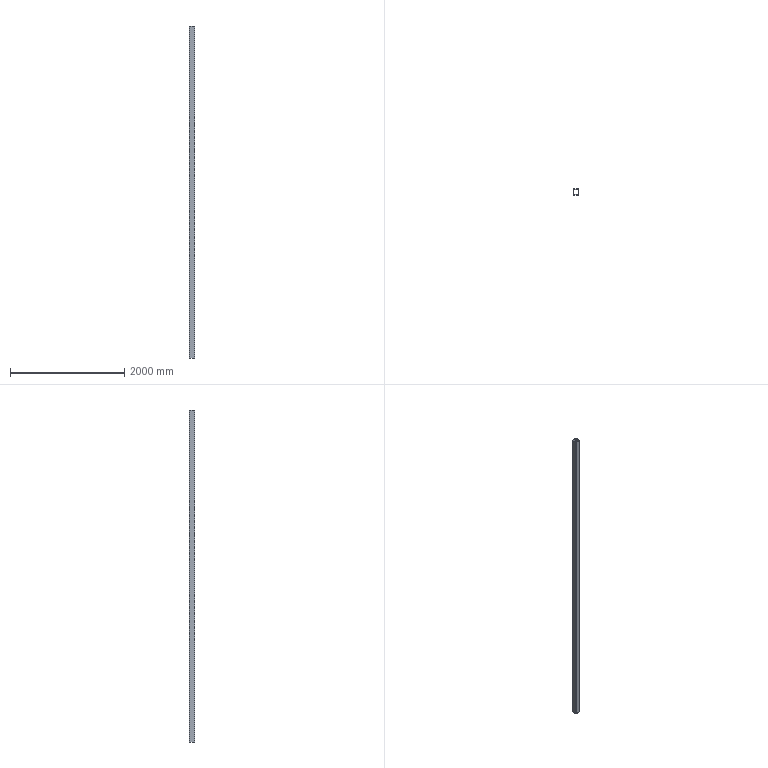Part | SolidWorks | features Extrusion 1 | 1 solid | 18 faces | box 100 x 100 x 5800 mm | volume 10646593 mm3 | plane 10 | cylinder 8 | commonest cylinder face diameters 10 x4 20 x4
STEP:
#1=CARTESIAN_POINT('',(90.,0.,5800.));
#2=VERTEX_POINT('',#1);
#3=CARTESIAN_POINT('',(100.,10.,5800.));
#4=VERTEX_POINT('',#3);
#5=CARTESIAN_POINT('',(90.,10.,5800.));
#6=DIRECTION('',(0.,0.,1.));
#7=DIRECTION('',(-1.,0.,0.));
#8=AXIS2_PLACEMENT_3D('',#5,#6,#7);
#9=CIRCLE('',#8,10.);
#10=EDGE_CURVE('',#2,#4,#9,.T.);
#11=ORIENTED_EDGE('',*,*,#10,.T.);
#12=CARTESIAN_POINT('',(100.,90.,5800.));
#13=VERTEX_POINT('',#12);
#14=CARTESIAN_POINT('',(100.,10.,5800.));
#15=DIRECTION('',(0.,1.,0.));
#16=VECTOR('',#15,1000.);
#17=LINE('',#14,#16);
#18=EDGE_CURVE('',#4,#13,#17,.T.);
#19=ORIENTED_EDGE('',*,*,#18,.T.);
#20=CARTESIAN_POINT('',(90.,100.,5800.));
#21=VERTEX_POINT('',#20);
#22=CARTESIAN_POINT('',(90.,90.,5800.));
#23=DIRECTION('',(0.,0.,1.));
#24=DIRECTION('',(1.,0.,0.));
#25=AXIS2_PLACEMENT_3D('',#22,#23,#24);
#26=CIRCLE('',#25,10.);
#27=EDGE_CURVE('',#13,#21,#26,.T.);
#28=ORIENTED_EDGE('',*,*,#27,.T.);
#29=CARTESIAN_POINT('',(10.,100.,5800.));
#30=VERTEX_POINT('',#29);
#31=CARTESIAN_POINT('',(10.,100.,5800.));
#32=DIRECTION('',(-1.,0.,0.));
#33=VECTOR('',#32,1000.);
#34=LINE('',#31,#33);
#35=EDGE_CURVE('',#21,#30,#34,.T.);
#36=ORIENTED_EDGE('',*,*,#35,.T.);
#37=CARTESIAN_POINT('',(0.,90.,5800.));
#38=VERTEX_POINT('',#37);
#39=CARTESIAN_POINT('',(10.,90.,5800.));
#40=DIRECTION('',(0.,0.,1.));
#41=DIRECTION('',(-1.,0.,0.));
#42=AXIS2_PLACEMENT_3D('',#39,#40,#41);
#43=CIRCLE('',#42,10.);
#44=EDGE_CURVE('',#30,#38,#43,.T.);
#45=ORIENTED_EDGE('',*,*,#44,.T.);
#46=CARTESIAN_POINT('',(0.,10.,5800.));
#47=VERTEX_POINT('',#46);
#48=CARTESIAN_POINT('',(0.,10.,5800.));
#49=DIRECTION('',(0.,-1.,0.));
#50=VECTOR('',#49,1000.);
#51=LINE('',#48,#50);
#52=EDGE_CURVE('',#38,#47,#51,.T.);
#53=ORIENTED_EDGE('',*,*,#52,.T.);
#54=CARTESIAN_POINT('',(10.,0.,5800.));
#55=VERTEX_POINT('',#54);
#56=CARTESIAN_POINT('',(10.,10.,5800.));
#57=DIRECTION('',(0.,0.,1.));
#58=DIRECTION('',(-1.,0.,0.));
#59=AXIS2_PLACEMENT_3D('',#56,#57,#58);
#60=CIRCLE('',#59,10.);
#61=EDGE_CURVE('',#47,#55,#60,.T.);
#62=ORIENTED_EDGE('',*,*,#61,.T.);
#63=CARTESIAN_POINT('',(10.,0.,5800.));
#64=DIRECTION('',(1.,0.,0.));
#65=VECTOR('',#64,1000.);
#66=LINE('',#63,#65);
#67=EDGE_CURVE('',#55,#2,#66,.T.);
#68=ORIENTED_EDGE('',*,*,#67,.T.);
#69=EDGE_LOOP('',(#11,#19,#28,#36,#45,#53,#62,#68));
#70=FACE_OUTER_BOUND('',#69,.T.);
#71=CARTESIAN_POINT('',(10.,95.,5800.));
#72=VERTEX_POINT('',#71);
#73=CARTESIAN_POINT('',(5.,90.,5800.));
#74=VERTEX_POINT('',#73);
#75=CARTESIAN_POINT('',(10.,90.,5800.));
#76=DIRECTION('',(0.,0.,1.));
#77=DIRECTION('',(-1.,0.,0.));
#78=AXIS2_PLACEMENT_3D('',#75,#76,#77);
#79=CIRCLE('',#78,5.);
#80=EDGE_CURVE('',#72,#74,#79,.T.);
#81=ORIENTED_EDGE('',*,*,#80,.F.);
#82=CARTESIAN_POINT('',(90.,95.,5800.));
#83=VERTEX_POINT('',#82);
#84=CARTESIAN_POINT('',(10.,95.,5800.));
#85=DIRECTION('',(-1.,0.,0.));
#86=VECTOR('',#85,1000.);
#87=LINE('',#84,#86);
#88=EDGE_CURVE('',#83,#72,#87,.T.);
#89=ORIENTED_EDGE('',*,*,#88,.F.);
#90=CARTESIAN_POINT('',(95.,90.,5800.));
#91=VERTEX_POINT('',#90);
#92=CARTESIAN_POINT('',(90.,90.,5800.));
#93=DIRECTION('',(0.,0.,1.));
#94=DIRECTION('',(1.,0.,0.));
#95=AXIS2_PLACEMENT_3D('',#92,#93,#94);
#96=CIRCLE('',#95,5.);
#97=EDGE_CURVE('',#91,#83,#96,.T.);
#98=ORIENTED_EDGE('',*,*,#97,.F.);
#99=CARTESIAN_POINT('',(95.,10.,5800.));
#100=VERTEX_POINT('',#99);
#101=CARTESIAN_POINT('',(95.,10.,5800.));
#102=DIRECTION('',(0.,1.,0.));
#103=VECTOR('',#102,1000.);
#104=LINE('',#101,#103);
#105=EDGE_CURVE('',#100,#91,#104,.T.);
#106=ORIENTED_EDGE('',*,*,#105,.F.);
#107=CARTESIAN_POINT('',(90.,5.,5800.));
#108=VERTEX_POINT('',#107);
#109=CARTESIAN_POINT('',(90.,10.,5800.));
#110=DIRECTION('',(0.,0.,1.));
#111=DIRECTION('',(-1.,0.,0.));
#112=AXIS2_PLACEMENT_3D('',#109,#110,#111);
#113=CIRCLE('',#112,5.);
#114=EDGE_CURVE('',#108,#100,#113,.T.);
#115=ORIENTED_EDGE('',*,*,#114,.F.);
#116=CARTESIAN_POINT('',(10.,5.,5800.));
#117=VERTEX_POINT('',#116);
#118=CARTESIAN_POINT('',(10.,5.,5800.));
#119=DIRECTION('',(1.,0.,0.));
#120=VECTOR('',#119,1000.);
#121=LINE('',#118,#120);
#122=EDGE_CURVE('',#117,#108,#121,.T.);
#123=ORIENTED_EDGE('',*,*,#122,.F.);
#124=CARTESIAN_POINT('',(5.,10.,5800.));
#125=VERTEX_POINT('',#124);
#126=CARTESIAN_POINT('',(10.,10.,5800.));
#127=DIRECTION('',(0.,0.,1.));
#128=DIRECTION('',(-1.,0.,0.));
#129=AXIS2_PLACEMENT_3D('',#126,#127,#128);
#130=CIRCLE('',#129,5.);
#131=EDGE_CURVE('',#125,#117,#130,.T.);
#132=ORIENTED_EDGE('',*,*,#131,.F.);
#133=CARTESIAN_POINT('',(5.,10.,5800.));
#134=DIRECTION('',(0.,-1.,0.));
#135=VECTOR('',#134,1000.);
#136=LINE('',#133,#135);
#137=EDGE_CURVE('',#74,#125,#136,.T.);
#138=ORIENTED_EDGE('',*,*,#137,.F.);
#139=EDGE_LOOP('',(#81,#89,#98,#106,#115,#123,#132,#138));
#140=FACE_BOUND('',#139,.T.);
#141=CARTESIAN_POINT('',(90.,10.,5800.));
#142=DIRECTION('',(0.,0.,-1.));
#143=DIRECTION('',(-1.,0.,0.));
#144=AXIS2_PLACEMENT_3D('',#141,#142,#143);
#145=PLANE('',#144);
#146=ADVANCED_FACE('',(#70,#140),#145,.F.);
#147=CARTESIAN_POINT('',(90.,0.,0.));
#148=VERTEX_POINT('',#147);
#149=CARTESIAN_POINT('',(100.,10.,0.));
#150=VERTEX_POINT('',#149);
#151=CARTESIAN_POINT('',(90.,10.,0.));
#152=DIRECTION('',(0.,0.,1.));
#153=DIRECTION('',(-1.,0.,0.));
#154=AXIS2_PLACEMENT_3D('',#151,#152,#153);
#155=CIRCLE('',#154,10.);
#156=EDGE_CURVE('',#148,#150,#155,.T.);
#157=ORIENTED_EDGE('',*,*,#156,.F.);
#158=CARTESIAN_POINT('',(10.,0.,0.));
#159=VERTEX_POINT('',#158);
#160=CARTESIAN_POINT('',(10.,0.,0.));
#161=DIRECTION('',(1.,0.,0.));
#162=VECTOR('',#161,1000.);
#163=LINE('',#160,#162);
#164=EDGE_CURVE('',#159,#148,#163,.T.);
#165=ORIENTED_EDGE('',*,*,#164,.F.);
#166=CARTESIAN_POINT('',(0.,10.,0.));
#167=VERTEX_POINT('',#166);
#168=CARTESIAN_POINT('',(10.,10.,0.));
#169=DIRECTION('',(0.,0.,1.));
#170=DIRECTION('',(-1.,0.,0.));
#171=AXIS2_PLACEMENT_3D('',#168,#169,#170);
#172=CIRCLE('',#171,10.);
#173=EDGE_CURVE('',#167,#159,#172,.T.);
#174=ORIENTED_EDGE('',*,*,#173,.F.);
#175=CARTESIAN_POINT('',(0.,90.,0.));
#176=VERTEX_POINT('',#175);
#177=CARTESIAN_POINT('',(0.,10.,0.));
#178=DIRECTION('',(0.,-1.,0.));
#179=VECTOR('',#178,1000.);
#180=LINE('',#177,#179);
#181=EDGE_CURVE('',#176,#167,#180,.T.);
#182=ORIENTED_EDGE('',*,*,#181,.F.);
#183=CARTESIAN_POINT('',(10.,100.,0.));
#184=VERTEX_POINT('',#183);
#185=CARTESIAN_POINT('',(10.,90.,0.));
#186=DIRECTION('',(0.,0.,1.));
#187=DIRECTION('',(-1.,0.,0.));
#188=AXIS2_PLACEMENT_3D('',#185,#186,#187);
#189=CIRCLE('',#188,10.);
#190=EDGE_CURVE('',#184,#176,#189,.T.);
#191=ORIENTED_EDGE('',*,*,#190,.F.);
#192=CARTESIAN_POINT('',(90.,100.,0.));
#193=VERTEX_POINT('',#192);
#194=CARTESIAN_POINT('',(10.,100.,0.));
#195=DIRECTION('',(-1.,0.,0.));
#196=VECTOR('',#195,1000.);
#197=LINE('',#194,#196);
#198=EDGE_CURVE('',#193,#184,#197,.T.);
#199=ORIENTED_EDGE('',*,*,#198,.F.);
#200=CARTESIAN_POINT('',(100.,90.,0.));
#201=VERTEX_POINT('',#200);
#202=CARTESIAN_POINT('',(90.,90.,0.));
#203=DIRECTION('',(0.,0.,1.));
#204=DIRECTION('',(1.,0.,0.));
#205=AXIS2_PLACEMENT_3D('',#202,#203,#204);
#206=CIRCLE('',#205,10.);
#207=EDGE_CURVE('',#201,#193,#206,.T.);
#208=ORIENTED_EDGE('',*,*,#207,.F.);
#209=CARTESIAN_POINT('',(100.,10.,0.));
#210=DIRECTION('',(0.,1.,0.));
#211=VECTOR('',#210,1000.);
#212=LINE('',#209,#211);
#213=EDGE_CURVE('',#150,#201,#212,.T.);
#214=ORIENTED_EDGE('',*,*,#213,.F.);
#215=EDGE_LOOP('',(#157,#165,#174,#182,#191,#199,#208,#214));
#216=FACE_OUTER_BOUND('',#215,.T.);
#217=CARTESIAN_POINT('',(90.,95.,0.));
#218=VERTEX_POINT('',#217);
#219=CARTESIAN_POINT('',(10.,95.,0.));
#220=VERTEX_POINT('',#219);
#221=CARTESIAN_POINT('',(10.,95.,0.));
#222=DIRECTION('',(-1.,0.,0.));
#223=VECTOR('',#222,1000.);
#224=LINE('',#221,#223);
#225=EDGE_CURVE('',#218,#220,#224,.T.);
#226=ORIENTED_EDGE('',*,*,#225,.T.);
#227=CARTESIAN_POINT('',(5.,90.,0.));
#228=VERTEX_POINT('',#227);
#229=CARTESIAN_POINT('',(10.,90.,0.));
#230=DIRECTION('',(0.,0.,1.));
#231=DIRECTION('',(-1.,0.,0.));
#232=AXIS2_PLACEMENT_3D('',#229,#230,#231);
#233=CIRCLE('',#232,5.);
#234=EDGE_CURVE('',#220,#228,#233,.T.);
#235=ORIENTED_EDGE('',*,*,#234,.T.);
#236=CARTESIAN_POINT('',(5.,10.,0.));
#237=VERTEX_POINT('',#236);
#238=CARTESIAN_POINT('',(5.,10.,0.));
#239=DIRECTION('',(0.,-1.,0.));
#240=VECTOR('',#239,1000.);
#241=LINE('',#238,#240);
#242=EDGE_CURVE('',#228,#237,#241,.T.);
#243=ORIENTED_EDGE('',*,*,#242,.T.);
#244=CARTESIAN_POINT('',(10.,5.,0.));
#245=VERTEX_POINT('',#244);
#246=CARTESIAN_POINT('',(10.,10.,0.));
#247=DIRECTION('',(0.,0.,1.));
#248=DIRECTION('',(-1.,0.,0.));
#249=AXIS2_PLACEMENT_3D('',#246,#247,#248);
#250=CIRCLE('',#249,5.);
#251=EDGE_CURVE('',#237,#245,#250,.T.);
#252=ORIENTED_EDGE('',*,*,#251,.T.);
#253=CARTESIAN_POINT('',(90.,5.,0.));
#254=VERTEX_POINT('',#253);
#255=CARTESIAN_POINT('',(10.,5.,0.));
#256=DIRECTION('',(1.,0.,0.));
#257=VECTOR('',#256,1000.);
#258=LINE('',#255,#257);
#259=EDGE_CURVE('',#245,#254,#258,.T.);
#260=ORIENTED_EDGE('',*,*,#259,.T.);
#261=CARTESIAN_POINT('',(95.,10.,0.));
#262=VERTEX_POINT('',#261);
#263=CARTESIAN_POINT('',(90.,10.,0.));
#264=DIRECTION('',(0.,0.,1.));
#265=DIRECTION('',(-1.,0.,0.));
#266=AXIS2_PLACEMENT_3D('',#263,#264,#265);
#267=CIRCLE('',#266,5.);
#268=EDGE_CURVE('',#254,#262,#267,.T.);
#269=ORIENTED_EDGE('',*,*,#268,.T.);
#270=CARTESIAN_POINT('',(95.,90.,0.));
#271=VERTEX_POINT('',#270);
#272=CARTESIAN_POINT('',(95.,10.,0.));
#273=DIRECTION('',(0.,1.,0.));
#274=VECTOR('',#273,1000.);
#275=LINE('',#272,#274);
#276=EDGE_CURVE('',#262,#271,#275,.T.);
#277=ORIENTED_EDGE('',*,*,#276,.T.);
#278=CARTESIAN_POINT('',(90.,90.,0.));
#279=DIRECTION('',(0.,0.,1.));
#280=DIRECTION('',(1.,0.,0.));
#281=AXIS2_PLACEMENT_3D('',#278,#279,#280);
#282=CIRCLE('',#281,5.);
#283=EDGE_CURVE('',#271,#218,#282,.T.);
#284=ORIENTED_EDGE('',*,*,#283,.T.);
#285=EDGE_LOOP('',(#226,#235,#243,#252,#260,#269,#277,#284));
#286=FACE_BOUND('',#285,.T.);
#287=CARTESIAN_POINT('',(90.,10.,0.));
#288=DIRECTION('',(0.,0.,-1.));
#289=DIRECTION('',(-1.,0.,0.));
#290=AXIS2_PLACEMENT_3D('',#287,#288,#289);
#291=PLANE('',#290);
#292=ADVANCED_FACE('',(#216,#286),#291,.T.);
#293=ORIENTED_EDGE('',*,*,#156,.T.);
#294=CARTESIAN_POINT('',(100.,10.,5800.));
#295=DIRECTION('',(0.,0.,-1.));
#296=VECTOR('',#295,1000.);
#297=LINE('',#294,#296);
#298=EDGE_CURVE('',#4,#150,#297,.T.);
#299=ORIENTED_EDGE('',*,*,#298,.F.);
#300=ORIENTED_EDGE('',*,*,#10,.F.);
#301=CARTESIAN_POINT('',(90.,0.,5800.));
#302=DIRECTION('',(0.,0.,-1.));
#303=VECTOR('',#302,1000.);
#304=LINE('',#301,#303);
#305=EDGE_CURVE('',#2,#148,#304,.T.);
#306=ORIENTED_EDGE('',*,*,#305,.T.);
#307=EDGE_LOOP('',(#293,#299,#300,#306));
#308=FACE_OUTER_BOUND('',#307,.T.);
#309=CARTESIAN_POINT('',(90.,10.,5800.));
#310=DIRECTION('',(0.,0.,-1.));
#311=DIRECTION('',(-1.,0.,0.));
#312=AXIS2_PLACEMENT_3D('',#309,#310,#311);
#313=CYLINDRICAL_SURFACE('',#312,10.);
#314=ADVANCED_FACE('',(#308),#313,.T.);
#315=ORIENTED_EDGE('',*,*,#213,.T.);
#316=CARTESIAN_POINT('',(100.,90.,5800.));
#317=DIRECTION('',(0.,0.,-1.));
#318=VECTOR('',#317,1000.);
#319=LINE('',#316,#318);
#320=EDGE_CURVE('',#13,#201,#319,.T.);
#321=ORIENTED_EDGE('',*,*,#320,.F.);
#322=ORIENTED_EDGE('',*,*,#18,.F.);
#323=ORIENTED_EDGE('',*,*,#298,.T.);
#324=EDGE_LOOP('',(#315,#321,#322,#323));
#325=FACE_OUTER_BOUND('',#324,.T.);
#326=CARTESIAN_POINT('',(100.,10.,5800.));
#327=DIRECTION('',(-1.,0.,0.));
#328=DIRECTION('',(0.,0.,1.));
#329=AXIS2_PLACEMENT_3D('',#326,#327,#328);
#330=PLANE('',#329);
#331=ADVANCED_FACE('',(#325),#330,.F.);
#332=ORIENTED_EDGE('',*,*,#207,.T.);
#333=CARTESIAN_POINT('',(90.,100.,5800.));
#334=DIRECTION('',(0.,0.,-1.));
#335=VECTOR('',#334,1000.);
#336=LINE('',#333,#335);
#337=EDGE_CURVE('',#21,#193,#336,.T.);
#338=ORIENTED_EDGE('',*,*,#337,.F.);
#339=ORIENTED_EDGE('',*,*,#27,.F.);
#340=ORIENTED_EDGE('',*,*,#320,.T.);
#341=EDGE_LOOP('',(#332,#338,#339,#340));
#342=FACE_OUTER_BOUND('',#341,.T.);
#343=CARTESIAN_POINT('',(90.,90.,5800.));
#344=DIRECTION('',(0.,0.,-1.));
#345=DIRECTION('',(-1.,0.,0.));
#346=AXIS2_PLACEMENT_3D('',#343,#344,#345);
#347=CYLINDRICAL_SURFACE('',#346,10.);
#348=ADVANCED_FACE('',(#342),#347,.T.);
#349=ORIENTED_EDGE('',*,*,#198,.T.);
#350=CARTESIAN_POINT('',(10.,100.,5800.));
#351=DIRECTION('',(0.,0.,-1.));
#352=VECTOR('',#351,1000.);
#353=LINE('',#350,#352);
#354=EDGE_CURVE('',#30,#184,#353,.T.);
#355=ORIENTED_EDGE('',*,*,#354,.F.);
#356=ORIENTED_EDGE('',*,*,#35,.F.);
#357=ORIENTED_EDGE('',*,*,#337,.T.);
#358=EDGE_LOOP('',(#349,#355,#356,#357));
#359=FACE_OUTER_BOUND('',#358,.T.);
#360=CARTESIAN_POINT('',(10.,100.,5800.));
#361=DIRECTION('',(0.,-1.,0.));
#362=DIRECTION('',(0.,0.,-1.));
#363=AXIS2_PLACEMENT_3D('',#360,#361,#362);
#364=PLANE('',#363);
#365=ADVANCED_FACE('',(#359),#364,.F.);
#366=ORIENTED_EDGE('',*,*,#190,.T.);
#367=CARTESIAN_POINT('',(0.,90.,5800.));
#368=DIRECTION('',(0.,0.,-1.));
#369=VECTOR('',#368,1000.);
#370=LINE('',#367,#369);
#371=EDGE_CURVE('',#38,#176,#370,.T.);
#372=ORIENTED_EDGE('',*,*,#371,.F.);
#373=ORIENTED_EDGE('',*,*,#44,.F.);
#374=ORIENTED_EDGE('',*,*,#354,.T.);
#375=EDGE_LOOP('',(#366,#372,#373,#374));
#376=FACE_OUTER_BOUND('',#375,.T.);
#377=CARTESIAN_POINT('',(10.,90.,5800.));
#378=DIRECTION('',(0.,0.,-1.));
#379=DIRECTION('',(-1.,0.,0.));
#380=AXIS2_PLACEMENT_3D('',#377,#378,#379);
#381=CYLINDRICAL_SURFACE('',#380,10.);
#382=ADVANCED_FACE('',(#376),#381,.T.);
#383=ORIENTED_EDGE('',*,*,#181,.T.);
#384=CARTESIAN_POINT('',(0.,10.,5800.));
#385=DIRECTION('',(0.,0.,-1.));
#386=VECTOR('',#385,1000.);
#387=LINE('',#384,#386);
#388=EDGE_CURVE('',#47,#167,#387,.T.);
#389=ORIENTED_EDGE('',*,*,#388,.F.);
#390=ORIENTED_EDGE('',*,*,#52,.F.);
#391=ORIENTED_EDGE('',*,*,#371,.T.);
#392=EDGE_LOOP('',(#383,#389,#390,#391));
#393=FACE_OUTER_BOUND('',#392,.T.);
#394=CARTESIAN_POINT('',(0.,10.,5800.));
#395=DIRECTION('',(1.,0.,0.));
#396=DIRECTION('',(0.,1.,0.));
#397=AXIS2_PLACEMENT_3D('',#394,#395,#396);
#398=PLANE('',#397);
#399=ADVANCED_FACE('',(#393),#398,.F.);
#400=ORIENTED_EDGE('',*,*,#173,.T.);
#401=CARTESIAN_POINT('',(10.,0.,5800.));
#402=DIRECTION('',(0.,0.,-1.));
#403=VECTOR('',#402,1000.);
#404=LINE('',#401,#403);
#405=EDGE_CURVE('',#55,#159,#404,.T.);
#406=ORIENTED_EDGE('',*,*,#405,.F.);
#407=ORIENTED_EDGE('',*,*,#61,.F.);
#408=ORIENTED_EDGE('',*,*,#388,.T.);
#409=EDGE_LOOP('',(#400,#406,#407,#408));
#410=FACE_OUTER_BOUND('',#409,.T.);
#411=CARTESIAN_POINT('',(10.,10.,5800.));
#412=DIRECTION('',(0.,0.,-1.));
#413=DIRECTION('',(-1.,0.,0.));
#414=AXIS2_PLACEMENT_3D('',#411,#412,#413);
#415=CYLINDRICAL_SURFACE('',#414,10.);
#416=ADVANCED_FACE('',(#410),#415,.T.);
#417=ORIENTED_EDGE('',*,*,#164,.T.);
#418=ORIENTED_EDGE('',*,*,#305,.F.);
#419=ORIENTED_EDGE('',*,*,#67,.F.);
#420=ORIENTED_EDGE('',*,*,#405,.T.);
#421=EDGE_LOOP('',(#417,#418,#419,#420));
#422=FACE_OUTER_BOUND('',#421,.T.);
#423=CARTESIAN_POINT('',(10.,0.,5800.));
#424=DIRECTION('',(0.,1.,0.));
#425=DIRECTION('',(0.,0.,1.));
#426=AXIS2_PLACEMENT_3D('',#423,#424,#425);
#427=PLANE('',#426);
#428=ADVANCED_FACE('',(#422),#427,.F.);
#429=ORIENTED_EDGE('',*,*,#234,.F.);
#430=CARTESIAN_POINT('',(10.,95.,5800.));
#431=DIRECTION('',(0.,0.,-1.));
#432=VECTOR('',#431,1000.);
#433=LINE('',#430,#432);
#434=EDGE_CURVE('',#72,#220,#433,.T.);
#435=ORIENTED_EDGE('',*,*,#434,.F.);
#436=ORIENTED_EDGE('',*,*,#80,.T.);
#437=CARTESIAN_POINT('',(5.,90.,5800.));
#438=DIRECTION('',(0.,0.,-1.));
#439=VECTOR('',#438,1000.);
#440=LINE('',#437,#439);
#441=EDGE_CURVE('',#74,#228,#440,.T.);
#442=ORIENTED_EDGE('',*,*,#441,.T.);
#443=EDGE_LOOP('',(#429,#435,#436,#442));
#444=FACE_OUTER_BOUND('',#443,.T.);
#445=CARTESIAN_POINT('',(10.,90.,5800.));
#446=DIRECTION('',(0.,0.,-1.));
#447=DIRECTION('',(-1.,0.,0.));
#448=AXIS2_PLACEMENT_3D('',#445,#446,#447);
#449=CYLINDRICAL_SURFACE('',#448,5.);
#450=ADVANCED_FACE('',(#444),#449,.F.);
#451=ORIENTED_EDGE('',*,*,#242,.F.);
#452=ORIENTED_EDGE('',*,*,#441,.F.);
#453=ORIENTED_EDGE('',*,*,#137,.T.);
#454=CARTESIAN_POINT('',(5.,10.,5800.));
#455=DIRECTION('',(0.,0.,-1.));
#456=VECTOR('',#455,1000.);
#457=LINE('',#454,#456);
#458=EDGE_CURVE('',#125,#237,#457,.T.);
#459=ORIENTED_EDGE('',*,*,#458,.T.);
#460=EDGE_LOOP('',(#451,#452,#453,#459));
#461=FACE_OUTER_BOUND('',#460,.T.);
#462=CARTESIAN_POINT('',(5.,10.,5800.));
#463=DIRECTION('',(1.,0.,0.));
#464=DIRECTION('',(0.,1.,0.));
#465=AXIS2_PLACEMENT_3D('',#462,#463,#464);
#466=PLANE('',#465);
#467=ADVANCED_FACE('',(#461),#466,.T.);
#468=ORIENTED_EDGE('',*,*,#251,.F.);
#469=ORIENTED_EDGE('',*,*,#458,.F.);
#470=ORIENTED_EDGE('',*,*,#131,.T.);
#471=CARTESIAN_POINT('',(10.,5.,5800.));
#472=DIRECTION('',(0.,0.,-1.));
#473=VECTOR('',#472,1000.);
#474=LINE('',#471,#473);
#475=EDGE_CURVE('',#117,#245,#474,.T.);
#476=ORIENTED_EDGE('',*,*,#475,.T.);
#477=EDGE_LOOP('',(#468,#469,#470,#476));
#478=FACE_OUTER_BOUND('',#477,.T.);
#479=CARTESIAN_POINT('',(10.,10.,5800.));
#480=DIRECTION('',(0.,0.,-1.));
#481=DIRECTION('',(-1.,0.,0.));
#482=AXIS2_PLACEMENT_3D('',#479,#480,#481);
#483=CYLINDRICAL_SURFACE('',#482,5.);
#484=ADVANCED_FACE('',(#478),#483,.F.);
#485=ORIENTED_EDGE('',*,*,#259,.F.);
#486=ORIENTED_EDGE('',*,*,#475,.F.);
#487=ORIENTED_EDGE('',*,*,#122,.T.);
#488=CARTESIAN_POINT('',(90.,5.,5800.));
#489=DIRECTION('',(0.,0.,-1.));
#490=VECTOR('',#489,1000.);
#491=LINE('',#488,#490);
#492=EDGE_CURVE('',#108,#254,#491,.T.);
#493=ORIENTED_EDGE('',*,*,#492,.T.);
#494=EDGE_LOOP('',(#485,#486,#487,#493));
#495=FACE_OUTER_BOUND('',#494,.T.);
#496=CARTESIAN_POINT('',(10.,5.,5800.));
#497=DIRECTION('',(0.,1.,0.));
#498=DIRECTION('',(0.,0.,1.));
#499=AXIS2_PLACEMENT_3D('',#496,#497,#498);
#500=PLANE('',#499);
#501=ADVANCED_FACE('',(#495),#500,.T.);
#502=ORIENTED_EDGE('',*,*,#268,.F.);
#503=ORIENTED_EDGE('',*,*,#492,.F.);
#504=ORIENTED_EDGE('',*,*,#114,.T.);
#505=CARTESIAN_POINT('',(95.,10.,5800.));
#506=DIRECTION('',(0.,0.,-1.));
#507=VECTOR('',#506,1000.);
#508=LINE('',#505,#507);
#509=EDGE_CURVE('',#100,#262,#508,.T.);
#510=ORIENTED_EDGE('',*,*,#509,.T.);
#511=EDGE_LOOP('',(#502,#503,#504,#510));
#512=FACE_OUTER_BOUND('',#511,.T.);
#513=CARTESIAN_POINT('',(90.,10.,5800.));
#514=DIRECTION('',(0.,0.,-1.));
#515=DIRECTION('',(-1.,0.,0.));
#516=AXIS2_PLACEMENT_3D('',#513,#514,#515);
#517=CYLINDRICAL_SURFACE('',#516,5.);
#518=ADVANCED_FACE('',(#512),#517,.F.);
#519=ORIENTED_EDGE('',*,*,#276,.F.);
#520=ORIENTED_EDGE('',*,*,#509,.F.);
#521=ORIENTED_EDGE('',*,*,#105,.T.);
#522=CARTESIAN_POINT('',(95.,90.,5800.));
#523=DIRECTION('',(0.,0.,-1.));
#524=VECTOR('',#523,1000.);
#525=LINE('',#522,#524);
#526=EDGE_CURVE('',#91,#271,#525,.T.);
#527=ORIENTED_EDGE('',*,*,#526,.T.);
#528=EDGE_LOOP('',(#519,#520,#521,#527));
#529=FACE_OUTER_BOUND('',#528,.T.);
#530=CARTESIAN_POINT('',(95.,10.,5800.));
#531=DIRECTION('',(-1.,0.,0.));
#532=DIRECTION('',(0.,0.,1.));
#533=AXIS2_PLACEMENT_3D('',#530,#531,#532);
#534=PLANE('',#533);
#535=ADVANCED_FACE('',(#529),#534,.T.);
#536=ORIENTED_EDGE('',*,*,#283,.F.);
#537=ORIENTED_EDGE('',*,*,#526,.F.);
#538=ORIENTED_EDGE('',*,*,#97,.T.);
#539=CARTESIAN_POINT('',(90.,95.,5800.));
#540=DIRECTION('',(0.,0.,-1.));
#541=VECTOR('',#540,1000.);
#542=LINE('',#539,#541);
#543=EDGE_CURVE('',#83,#218,#542,.T.);
#544=ORIENTED_EDGE('',*,*,#543,.T.);
#545=EDGE_LOOP('',(#536,#537,#538,#544));
#546=FACE_OUTER_BOUND('',#545,.T.);
#547=CARTESIAN_POINT('',(90.,90.,5800.));
#548=DIRECTION('',(0.,0.,-1.));
#549=DIRECTION('',(-1.,0.,0.));
#550=AXIS2_PLACEMENT_3D('',#547,#548,#549);
#551=CYLINDRICAL_SURFACE('',#550,5.);
#552=ADVANCED_FACE('',(#546),#551,.F.);
#553=ORIENTED_EDGE('',*,*,#225,.F.);
#554=ORIENTED_EDGE('',*,*,#543,.F.);
#555=ORIENTED_EDGE('',*,*,#88,.T.);
#556=ORIENTED_EDGE('',*,*,#434,.T.);
#557=EDGE_LOOP('',(#553,#554,#555,#556));
#558=FACE_OUTER_BOUND('',#557,.T.);
#559=CARTESIAN_POINT('',(10.,95.,5800.));
#560=DIRECTION('',(0.,-1.,0.));
#561=DIRECTION('',(0.,0.,-1.));
#562=AXIS2_PLACEMENT_3D('',#559,#560,#561);
#563=PLANE('',#562);
#564=ADVANCED_FACE('',(#558),#563,.T.);
#565=CLOSED_SHELL('',(#146,#292,#314,#331,#348,#365,#382,#399,#416,#428,#450,#467,#484,#501,#518,#535,#552,#564));
#566=MANIFOLD_SOLID_BREP('',#565);
#567=CARTESIAN_POINT('',(0.,0.,0.));
#568=DIRECTION('',(0.,0.,1.));
#569=DIRECTION('',(1.,0.,0.));
#570=AXIS2_PLACEMENT_3D('',#567,#568,#569);
#571=(LENGTH_UNIT()NAMED_UNIT(*)SI_UNIT(.MILLI.,.METRE.));
#572=UNCERTAINTY_MEASURE_WITH_UNIT(LENGTH_MEASURE(0.00001),#571,'','');
#573=(NAMED_UNIT(*)PLANE_ANGLE_UNIT()SI_UNIT($,.RADIAN.));
#574=(NAMED_UNIT(*)SI_UNIT($,.STERADIAN.)SOLID_ANGLE_UNIT());
#575=(GEOMETRIC_REPRESENTATION_CONTEXT(3)GLOBAL_UNCERTAINTY_ASSIGNED_CONTEXT((#572))GLOBAL_UNIT_ASSIGNED_CONTEXT((#571,#573,#574))REPRESENTATION_CONTEXT('',''));
#576=ADVANCED_BREP_SHAPE_REPRESENTATION('',(#566,#570),#575);